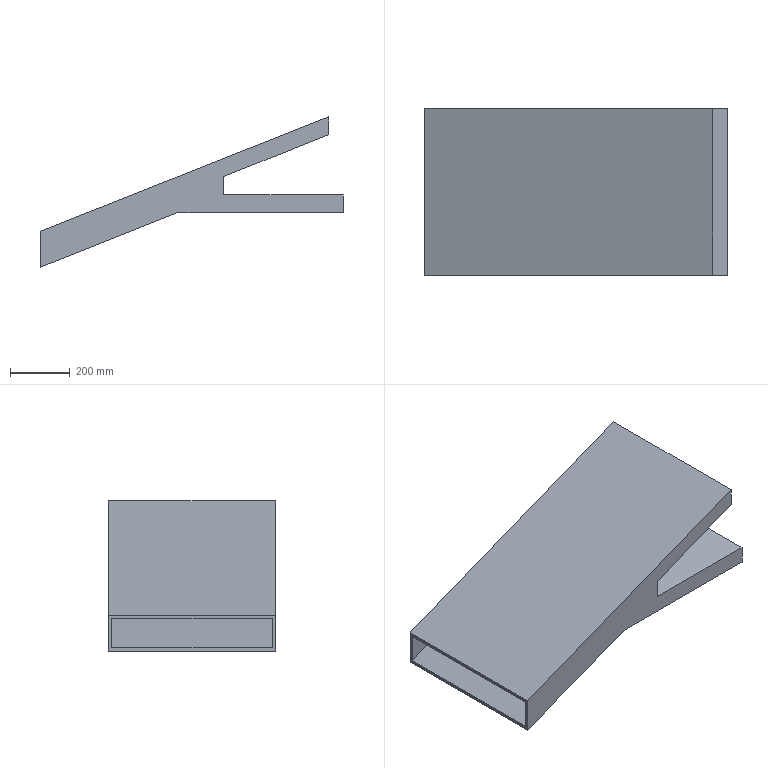Part | SolidWorks | features Extrusion 1, ICE 1, Shell 1 | 1 solid | 23 faces | box 1012 x 556 x 502.062 mm | volume 17769290 mm3 | plane 23
STEP:
#1=CARTESIAN_POINT('',(500.,0.,0.));
#2=VERTEX_POINT('',#1);
#3=CARTESIAN_POINT('',(500.,0.,-60.));
#4=VERTEX_POINT('',#3);
#5=CARTESIAN_POINT('',(500.,0.,0.));
#6=DIRECTION('',(0.,0.,-1.));
#7=VECTOR('',#6,1000.);
#8=LINE('',#5,#7);
#9=EDGE_CURVE('',#2,#4,#8,.T.);
#10=ORIENTED_EDGE('',*,*,#9,.T.);
#11=CARTESIAN_POINT('',(500.,556.,-60.));
#12=VERTEX_POINT('',#11);
#13=CARTESIAN_POINT('',(500.,556.,-60.));
#14=DIRECTION('',(0.,-1.,0.));
#15=VECTOR('',#14,1000.);
#16=LINE('',#13,#15);
#17=EDGE_CURVE('',#12,#4,#16,.T.);
#18=ORIENTED_EDGE('',*,*,#17,.F.);
#19=CARTESIAN_POINT('',(500.,556.,0.));
#20=VERTEX_POINT('',#19);
#21=CARTESIAN_POINT('',(500.,556.,0.));
#22=DIRECTION('',(0.,0.,-1.));
#23=VECTOR('',#22,1000.);
#24=LINE('',#21,#23);
#25=EDGE_CURVE('',#20,#12,#24,.T.);
#26=ORIENTED_EDGE('',*,*,#25,.F.);
#27=CARTESIAN_POINT('',(500.,556.,0.));
#28=DIRECTION('',(0.,-1.,0.));
#29=VECTOR('',#28,1000.);
#30=LINE('',#27,#29);
#31=EDGE_CURVE('',#20,#2,#30,.T.);
#32=ORIENTED_EDGE('',*,*,#31,.T.);
#33=EDGE_LOOP('',(#10,#18,#26,#32));
#34=FACE_OUTER_BOUND('',#33,.T.);
#35=CARTESIAN_POINT('',(500.,10.,-10.));
#36=VERTEX_POINT('',#35);
#37=CARTESIAN_POINT('',(500.,10.,-50.));
#38=VERTEX_POINT('',#37);
#39=CARTESIAN_POINT('',(500.,10.,0.));
#40=DIRECTION('',(0.,0.,-1.));
#41=VECTOR('',#40,1000.);
#42=LINE('',#39,#41);
#43=EDGE_CURVE('',#36,#38,#42,.T.);
#44=ORIENTED_EDGE('',*,*,#43,.F.);
#45=CARTESIAN_POINT('',(500.,546.,-10.));
#46=VERTEX_POINT('',#45);
#47=CARTESIAN_POINT('',(500.,556.,-10.));
#48=DIRECTION('',(0.,-1.,0.));
#49=VECTOR('',#48,1000.);
#50=LINE('',#47,#49);
#51=EDGE_CURVE('',#46,#36,#50,.T.);
#52=ORIENTED_EDGE('',*,*,#51,.F.);
#53=CARTESIAN_POINT('',(500.,546.,-50.));
#54=VERTEX_POINT('',#53);
#55=CARTESIAN_POINT('',(500.,546.,0.));
#56=DIRECTION('',(0.,0.,-1.));
#57=VECTOR('',#56,1000.);
#58=LINE('',#55,#57);
#59=EDGE_CURVE('',#46,#54,#58,.T.);
#60=ORIENTED_EDGE('',*,*,#59,.T.);
#61=CARTESIAN_POINT('',(500.,556.,-50.));
#62=DIRECTION('',(0.,-1.,0.));
#63=VECTOR('',#62,1000.);
#64=LINE('',#61,#63);
#65=EDGE_CURVE('',#54,#38,#64,.T.);
#66=ORIENTED_EDGE('',*,*,#65,.T.);
#67=EDGE_LOOP('',(#44,#52,#60,#66));
#68=FACE_BOUND('',#67,.T.);
#69=CARTESIAN_POINT('',(500.,556.,0.));
#70=DIRECTION('',(-1.,0.,0.));
#71=DIRECTION('',(0.,0.,1.));
#72=AXIS2_PLACEMENT_3D('',#69,#70,#71);
#73=PLANE('',#72);
#74=ADVANCED_FACE('',(#34,#68),#73,.F.);
#75=CARTESIAN_POINT('',(-511.593,0.,-241.017));
#76=VERTEX_POINT('',#75);
#77=CARTESIAN_POINT('',(-511.593,0.,-121.017));
#78=VERTEX_POINT('',#77);
#79=CARTESIAN_POINT('',(-511.593,0.,-241.017));
#80=DIRECTION('',(0.,0.,1.));
#81=VECTOR('',#80,1000.);
#82=LINE('',#79,#81);
#83=EDGE_CURVE('',#76,#78,#82,.T.);
#84=ORIENTED_EDGE('',*,*,#83,.T.);
#85=CARTESIAN_POINT('',(-511.593,556.,-121.017));
#86=VERTEX_POINT('',#85);
#87=CARTESIAN_POINT('',(-511.593,556.,-121.017));
#88=DIRECTION('',(0.,-1.,0.));
#89=VECTOR('',#88,1000.);
#90=LINE('',#87,#89);
#91=EDGE_CURVE('',#86,#78,#90,.T.);
#92=ORIENTED_EDGE('',*,*,#91,.F.);
#93=CARTESIAN_POINT('',(-511.593,556.,-241.017));
#94=VERTEX_POINT('',#93);
#95=CARTESIAN_POINT('',(-511.593,556.,-241.017));
#96=DIRECTION('',(0.,0.,1.));
#97=VECTOR('',#96,1000.);
#98=LINE('',#95,#97);
#99=EDGE_CURVE('',#94,#86,#98,.T.);
#100=ORIENTED_EDGE('',*,*,#99,.F.);
#101=CARTESIAN_POINT('',(-511.593,556.,-241.017));
#102=DIRECTION('',(0.,-1.,0.));
#103=VECTOR('',#102,1000.);
#104=LINE('',#101,#103);
#105=EDGE_CURVE('',#94,#76,#104,.T.);
#106=ORIENTED_EDGE('',*,*,#105,.T.);
#107=EDGE_LOOP('',(#84,#92,#100,#106));
#108=FACE_OUTER_BOUND('',#107,.T.);
#109=CARTESIAN_POINT('',(-511.593,10.,-230.257));
#110=VERTEX_POINT('',#109);
#111=CARTESIAN_POINT('',(-511.593,10.,-131.777));
#112=VERTEX_POINT('',#111);
#113=CARTESIAN_POINT('',(-511.593,10.,-241.017));
#114=DIRECTION('',(0.,0.,1.));
#115=VECTOR('',#114,1000.);
#116=LINE('',#113,#115);
#117=EDGE_CURVE('',#110,#112,#116,.T.);
#118=ORIENTED_EDGE('',*,*,#117,.F.);
#119=CARTESIAN_POINT('',(-511.593,546.,-230.257));
#120=VERTEX_POINT('',#119);
#121=CARTESIAN_POINT('',(-511.593,556.,-230.257));
#122=DIRECTION('',(0.,-1.,0.));
#123=VECTOR('',#122,1000.);
#124=LINE('',#121,#123);
#125=EDGE_CURVE('',#120,#110,#124,.T.);
#126=ORIENTED_EDGE('',*,*,#125,.F.);
#127=CARTESIAN_POINT('',(-511.593,546.,-131.777));
#128=VERTEX_POINT('',#127);
#129=CARTESIAN_POINT('',(-511.593,546.,-241.017));
#130=DIRECTION('',(0.,0.,1.));
#131=VECTOR('',#130,1000.);
#132=LINE('',#129,#131);
#133=EDGE_CURVE('',#120,#128,#132,.T.);
#134=ORIENTED_EDGE('',*,*,#133,.T.);
#135=CARTESIAN_POINT('',(-511.593,556.,-131.777));
#136=DIRECTION('',(0.,-1.,0.));
#137=VECTOR('',#136,1000.);
#138=LINE('',#135,#137);
#139=EDGE_CURVE('',#128,#112,#138,.T.);
#140=ORIENTED_EDGE('',*,*,#139,.T.);
#141=EDGE_LOOP('',(#118,#126,#134,#140));
#142=FACE_BOUND('',#141,.T.);
#143=CARTESIAN_POINT('',(-511.593,556.,-241.017));
#144=DIRECTION('',(1.,0.,0.));
#145=DIRECTION('',(0.,0.,-1.));
#146=AXIS2_PLACEMENT_3D('',#143,#144,#145);
#147=PLANE('',#146);
#148=ADVANCED_FACE('',(#108,#142),#147,.F.);
#149=CARTESIAN_POINT('',(450.,0.,261.045));
#150=VERTEX_POINT('',#149);
#151=CARTESIAN_POINT('',(450.,0.,201.045));
#152=VERTEX_POINT('',#151);
#153=CARTESIAN_POINT('',(450.,0.,261.045));
#154=DIRECTION('',(0.,0.,-1.));
#155=VECTOR('',#154,1000.);
#156=LINE('',#153,#155);
#157=EDGE_CURVE('',#150,#152,#156,.T.);
#158=ORIENTED_EDGE('',*,*,#157,.T.);
#159=CARTESIAN_POINT('',(450.,556.,201.045));
#160=VERTEX_POINT('',#159);
#161=CARTESIAN_POINT('',(450.,556.,201.045));
#162=DIRECTION('',(0.,-1.,0.));
#163=VECTOR('',#162,1000.);
#164=LINE('',#161,#163);
#165=EDGE_CURVE('',#160,#152,#164,.T.);
#166=ORIENTED_EDGE('',*,*,#165,.F.);
#167=CARTESIAN_POINT('',(450.,556.,261.045));
#168=VERTEX_POINT('',#167);
#169=CARTESIAN_POINT('',(450.,556.,261.045));
#170=DIRECTION('',(0.,0.,-1.));
#171=VECTOR('',#170,1000.);
#172=LINE('',#169,#171);
#173=EDGE_CURVE('',#168,#160,#172,.T.);
#174=ORIENTED_EDGE('',*,*,#173,.F.);
#175=CARTESIAN_POINT('',(450.,556.,261.045));
#176=DIRECTION('',(0.,-1.,0.));
#177=VECTOR('',#176,1000.);
#178=LINE('',#175,#177);
#179=EDGE_CURVE('',#168,#150,#178,.T.);
#180=ORIENTED_EDGE('',*,*,#179,.T.);
#181=EDGE_LOOP('',(#158,#166,#174,#180));
#182=FACE_OUTER_BOUND('',#181,.T.);
#183=CARTESIAN_POINT('',(450.,10.,250.284));
#184=VERTEX_POINT('',#183);
#185=CARTESIAN_POINT('',(450.,10.,211.805));
#186=VERTEX_POINT('',#185);
#187=CARTESIAN_POINT('',(450.,10.,261.045));
#188=DIRECTION('',(0.,0.,-1.));
#189=VECTOR('',#188,1000.);
#190=LINE('',#187,#189);
#191=EDGE_CURVE('',#184,#186,#190,.T.);
#192=ORIENTED_EDGE('',*,*,#191,.F.);
#193=CARTESIAN_POINT('',(450.,546.,250.284));
#194=VERTEX_POINT('',#193);
#195=CARTESIAN_POINT('',(450.,556.,250.284));
#196=DIRECTION('',(0.,-1.,0.));
#197=VECTOR('',#196,1000.);
#198=LINE('',#195,#197);
#199=EDGE_CURVE('',#194,#184,#198,.T.);
#200=ORIENTED_EDGE('',*,*,#199,.F.);
#201=CARTESIAN_POINT('',(450.,546.,211.805));
#202=VERTEX_POINT('',#201);
#203=CARTESIAN_POINT('',(450.,546.,261.045));
#204=DIRECTION('',(0.,0.,-1.));
#205=VECTOR('',#204,1000.);
#206=LINE('',#203,#205);
#207=EDGE_CURVE('',#194,#202,#206,.T.);
#208=ORIENTED_EDGE('',*,*,#207,.T.);
#209=CARTESIAN_POINT('',(450.,556.,211.805));
#210=DIRECTION('',(0.,-1.,0.));
#211=VECTOR('',#210,1000.);
#212=LINE('',#209,#211);
#213=EDGE_CURVE('',#202,#186,#212,.T.);
#214=ORIENTED_EDGE('',*,*,#213,.T.);
#215=EDGE_LOOP('',(#192,#200,#208,#214));
#216=FACE_BOUND('',#215,.T.);
#217=CARTESIAN_POINT('',(450.,556.,261.045));
#218=DIRECTION('',(-1.,0.,0.));
#219=DIRECTION('',(0.,0.,1.));
#220=AXIS2_PLACEMENT_3D('',#217,#218,#219);
#221=PLANE('',#220);
#222=ADVANCED_FACE('',(#182,#216),#221,.F.);
#223=CARTESIAN_POINT('',(-56.,41.096,-60.));
#224=VERTEX_POINT('',#223);
#225=CARTESIAN_POINT('',(-56.,0.,-60.));
#226=VERTEX_POINT('',#225);
#227=CARTESIAN_POINT('',(-56.,556.,-60.));
#228=DIRECTION('',(0.,-1.,0.));
#229=VECTOR('',#228,1000.);
#230=LINE('',#227,#229);
#231=EDGE_CURVE('',#224,#226,#230,.T.);
#232=ORIENTED_EDGE('',*,*,#231,.F.);
#233=CARTESIAN_POINT('',(44.,41.096,-60.));
#234=VERTEX_POINT('',#233);
#235=CARTESIAN_POINT('',(-56.,41.096,-60.));
#236=DIRECTION('',(-1.,0.,0.));
#237=VECTOR('',#236,1000.);
#238=LINE('',#235,#237);
#239=EDGE_CURVE('',#234,#224,#238,.T.);
#240=ORIENTED_EDGE('',*,*,#239,.F.);
#241=CARTESIAN_POINT('',(44.,485.332,-60.));
#242=VERTEX_POINT('',#241);
#243=CARTESIAN_POINT('',(44.,41.096,-60.));
#244=DIRECTION('',(0.,-1.,0.));
#245=VECTOR('',#244,1000.);
#246=LINE('',#243,#245);
#247=EDGE_CURVE('',#242,#234,#246,.T.);
#248=ORIENTED_EDGE('',*,*,#247,.F.);
#249=CARTESIAN_POINT('',(-56.,485.332,-60.));
#250=VERTEX_POINT('',#249);
#251=CARTESIAN_POINT('',(-56.,485.332,-60.));
#252=DIRECTION('',(1.,0.,0.));
#253=VECTOR('',#252,1000.);
#254=LINE('',#251,#253);
#255=EDGE_CURVE('',#250,#242,#254,.T.);
#256=ORIENTED_EDGE('',*,*,#255,.F.);
#257=CARTESIAN_POINT('',(-56.,556.,-60.));
#258=VERTEX_POINT('',#257);
#259=CARTESIAN_POINT('',(-56.,556.,-60.));
#260=DIRECTION('',(0.,-1.,0.));
#261=VECTOR('',#260,1000.);
#262=LINE('',#259,#261);
#263=EDGE_CURVE('',#258,#250,#262,.T.);
#264=ORIENTED_EDGE('',*,*,#263,.F.);
#265=CARTESIAN_POINT('',(500.,556.,-60.));
#266=DIRECTION('',(-1.,0.,0.));
#267=VECTOR('',#266,1000.);
#268=LINE('',#265,#267);
#269=EDGE_CURVE('',#12,#258,#268,.T.);
#270=ORIENTED_EDGE('',*,*,#269,.F.);
#271=ORIENTED_EDGE('',*,*,#17,.T.);
#272=CARTESIAN_POINT('',(500.,0.,-60.));
#273=DIRECTION('',(-1.,0.,0.));
#274=VECTOR('',#273,1000.);
#275=LINE('',#272,#274);
#276=EDGE_CURVE('',#4,#226,#275,.T.);
#277=ORIENTED_EDGE('',*,*,#276,.T.);
#278=EDGE_LOOP('',(#232,#240,#248,#256,#264,#270,#271,#277));
#279=FACE_OUTER_BOUND('',#278,.T.);
#280=CARTESIAN_POINT('',(500.,556.,-60.));
#281=DIRECTION('',(0.,0.,1.));
#282=DIRECTION('',(1.,0.,0.));
#283=AXIS2_PLACEMENT_3D('',#280,#281,#282);
#284=PLANE('',#283);
#285=ADVANCED_FACE('',(#279),#284,.F.);
#286=CARTESIAN_POINT('',(-56.,0.,-60.));
#287=DIRECTION('',(-0.9293,0.,-0.3692));
#288=VECTOR('',#287,1000.);
#289=LINE('',#286,#288);
#290=EDGE_CURVE('',#226,#76,#289,.T.);
#291=ORIENTED_EDGE('',*,*,#290,.T.);
#292=ORIENTED_EDGE('',*,*,#105,.F.);
#293=CARTESIAN_POINT('',(-56.,556.,-60.));
#294=DIRECTION('',(-0.9293,0.,-0.3692));
#295=VECTOR('',#294,1000.);
#296=LINE('',#293,#295);
#297=EDGE_CURVE('',#258,#94,#296,.T.);
#298=ORIENTED_EDGE('',*,*,#297,.F.);
#299=ORIENTED_EDGE('',*,*,#263,.T.);
#300=CARTESIAN_POINT('',(-56.,41.096,-60.));
#301=DIRECTION('',(0.,1.,0.));
#302=VECTOR('',#301,1000.);
#303=LINE('',#300,#302);
#304=EDGE_CURVE('',#224,#250,#303,.T.);
#305=ORIENTED_EDGE('',*,*,#304,.F.);
#306=ORIENTED_EDGE('',*,*,#231,.T.);
#307=EDGE_LOOP('',(#291,#292,#298,#299,#305,#306));
#308=FACE_OUTER_BOUND('',#307,.T.);
#309=CARTESIAN_POINT('',(-56.,556.,-60.));
#310=DIRECTION('',(-0.3692,0.,0.9293));
#311=DIRECTION('',(0.9293,0.,0.3692));
#312=AXIS2_PLACEMENT_3D('',#309,#310,#311);
#313=PLANE('',#312);
#314=ADVANCED_FACE('',(#308),#313,.F.);
#315=CARTESIAN_POINT('',(-511.593,0.,-121.017));
#316=DIRECTION('',(0.9293,0.,0.3692));
#317=VECTOR('',#316,1000.);
#318=LINE('',#315,#317);
#319=EDGE_CURVE('',#78,#150,#318,.T.);
#320=ORIENTED_EDGE('',*,*,#319,.T.);
#321=ORIENTED_EDGE('',*,*,#179,.F.);
#322=CARTESIAN_POINT('',(-511.593,556.,-121.017));
#323=DIRECTION('',(0.9293,0.,0.3692));
#324=VECTOR('',#323,1000.);
#325=LINE('',#322,#324);
#326=EDGE_CURVE('',#86,#168,#325,.T.);
#327=ORIENTED_EDGE('',*,*,#326,.F.);
#328=ORIENTED_EDGE('',*,*,#91,.T.);
#329=EDGE_LOOP('',(#320,#321,#327,#328));
#330=FACE_OUTER_BOUND('',#329,.T.);
#331=CARTESIAN_POINT('',(-511.593,556.,-121.017));
#332=DIRECTION('',(0.3692,0.,-0.9293));
#333=DIRECTION('',(-0.9293,0.,-0.3692));
#334=AXIS2_PLACEMENT_3D('',#331,#332,#333);
#335=PLANE('',#334);
#336=ADVANCED_FACE('',(#330),#335,.F.);
#337=CARTESIAN_POINT('',(100.,0.,61.982));
#338=VERTEX_POINT('',#337);
#339=CARTESIAN_POINT('',(450.,0.,201.045));
#340=DIRECTION('',(-0.9293,0.,-0.3692));
#341=VECTOR('',#340,1000.);
#342=LINE('',#339,#341);
#343=EDGE_CURVE('',#152,#338,#342,.T.);
#344=ORIENTED_EDGE('',*,*,#343,.T.);
#345=CARTESIAN_POINT('',(100.,556.,61.982));
#346=VERTEX_POINT('',#345);
#347=CARTESIAN_POINT('',(100.,556.,61.982));
#348=DIRECTION('',(0.,-1.,0.));
#349=VECTOR('',#348,1000.);
#350=LINE('',#347,#349);
#351=EDGE_CURVE('',#346,#338,#350,.T.);
#352=ORIENTED_EDGE('',*,*,#351,.F.);
#353=CARTESIAN_POINT('',(450.,556.,201.045));
#354=DIRECTION('',(-0.9293,0.,-0.3692));
#355=VECTOR('',#354,1000.);
#356=LINE('',#353,#355);
#357=EDGE_CURVE('',#160,#346,#356,.T.);
#358=ORIENTED_EDGE('',*,*,#357,.F.);
#359=ORIENTED_EDGE('',*,*,#165,.T.);
#360=EDGE_LOOP('',(#344,#352,#358,#359));
#361=FACE_OUTER_BOUND('',#360,.T.);
#362=CARTESIAN_POINT('',(450.,556.,201.045));
#363=DIRECTION('',(-0.3692,0.,0.9293));
#364=DIRECTION('',(0.9293,0.,0.3692));
#365=AXIS2_PLACEMENT_3D('',#362,#363,#364);
#366=PLANE('',#365);
#367=ADVANCED_FACE('',(#361),#366,.F.);
#368=CARTESIAN_POINT('',(100.,0.,0.));
#369=VERTEX_POINT('',#368);
#370=CARTESIAN_POINT('',(100.,0.,0.));
#371=DIRECTION('',(0.,0.,-1.));
#372=VECTOR('',#371,1000.);
#373=LINE('',#370,#372);
#374=EDGE_CURVE('',#338,#369,#373,.T.);
#375=ORIENTED_EDGE('',*,*,#374,.T.);
#376=CARTESIAN_POINT('',(100.,556.,0.));
#377=VERTEX_POINT('',#376);
#378=CARTESIAN_POINT('',(100.,556.,0.));
#379=DIRECTION('',(0.,-1.,0.));
#380=VECTOR('',#379,1000.);
#381=LINE('',#378,#380);
#382=EDGE_CURVE('',#377,#369,#381,.T.);
#383=ORIENTED_EDGE('',*,*,#382,.F.);
#384=CARTESIAN_POINT('',(100.,556.,0.));
#385=DIRECTION('',(0.,0.,-1.));
#386=VECTOR('',#385,1000.);
#387=LINE('',#384,#386);
#388=EDGE_CURVE('',#346,#377,#387,.T.);
#389=ORIENTED_EDGE('',*,*,#388,.F.);
#390=ORIENTED_EDGE('',*,*,#351,.T.);
#391=EDGE_LOOP('',(#375,#383,#389,#390));
#392=FACE_OUTER_BOUND('',#391,.T.);
#393=CARTESIAN_POINT('',(100.,556.,0.));
#394=DIRECTION('',(-1.,0.,0.));
#395=DIRECTION('',(0.,0.,1.));
#396=AXIS2_PLACEMENT_3D('',#393,#394,#395);
#397=PLANE('',#396);
#398=ADVANCED_FACE('',(#392),#397,.F.);
#399=CARTESIAN_POINT('',(100.,0.,0.));
#400=DIRECTION('',(1.,0.,0.));
#401=VECTOR('',#400,1000.);
#402=LINE('',#399,#401);
#403=EDGE_CURVE('',#369,#2,#402,.T.);
#404=ORIENTED_EDGE('',*,*,#403,.T.);
#405=ORIENTED_EDGE('',*,*,#31,.F.);
#406=CARTESIAN_POINT('',(100.,556.,0.));
#407=DIRECTION('',(1.,0.,0.));
#408=VECTOR('',#407,1000.);
#409=LINE('',#406,#408);
#410=EDGE_CURVE('',#377,#20,#409,.T.);
#411=ORIENTED_EDGE('',*,*,#410,.F.);
#412=ORIENTED_EDGE('',*,*,#382,.T.);
#413=EDGE_LOOP('',(#404,#405,#411,#412));
#414=FACE_OUTER_BOUND('',#413,.T.);
#415=CARTESIAN_POINT('',(100.,556.,0.));
#416=DIRECTION('',(0.,0.,-1.));
#417=DIRECTION('',(-1.,0.,0.));
#418=AXIS2_PLACEMENT_3D('',#415,#416,#417);
#419=PLANE('',#418);
#420=ADVANCED_FACE('',(#414),#419,.F.);
#421=ORIENTED_EDGE('',*,*,#25,.T.);
#422=ORIENTED_EDGE('',*,*,#269,.T.);
#423=ORIENTED_EDGE('',*,*,#297,.T.);
#424=ORIENTED_EDGE('',*,*,#99,.T.);
#425=ORIENTED_EDGE('',*,*,#326,.T.);
#426=ORIENTED_EDGE('',*,*,#173,.T.);
#427=ORIENTED_EDGE('',*,*,#357,.T.);
#428=ORIENTED_EDGE('',*,*,#388,.T.);
#429=ORIENTED_EDGE('',*,*,#410,.T.);
#430=EDGE_LOOP('',(#421,#422,#423,#424,#425,#426,#427,#428,#429));
#431=FACE_OUTER_BOUND('',#430,.T.);
#432=CARTESIAN_POINT('',(0.,556.,0.));
#433=DIRECTION('',(0.,1.,0.));
#434=DIRECTION('',(0.,0.,1.));
#435=AXIS2_PLACEMENT_3D('',#432,#433,#434);
#436=PLANE('',#435);
#437=ADVANCED_FACE('',(#431),#436,.T.);
#438=ORIENTED_EDGE('',*,*,#9,.F.);
#439=ORIENTED_EDGE('',*,*,#403,.F.);
#440=ORIENTED_EDGE('',*,*,#374,.F.);
#441=ORIENTED_EDGE('',*,*,#343,.F.);
#442=ORIENTED_EDGE('',*,*,#157,.F.);
#443=ORIENTED_EDGE('',*,*,#319,.F.);
#444=ORIENTED_EDGE('',*,*,#83,.F.);
#445=ORIENTED_EDGE('',*,*,#290,.F.);
#446=ORIENTED_EDGE('',*,*,#276,.F.);
#447=EDGE_LOOP('',(#438,#439,#440,#441,#442,#443,#444,#445,#446));
#448=FACE_OUTER_BOUND('',#447,.T.);
#449=CARTESIAN_POINT('',(0.,0.,0.));
#450=DIRECTION('',(0.,1.,0.));
#451=DIRECTION('',(0.,0.,1.));
#452=AXIS2_PLACEMENT_3D('',#449,#450,#451);
#453=PLANE('',#452);
#454=ADVANCED_FACE('',(#448),#453,.F.);
#455=CARTESIAN_POINT('',(-56.,485.332,-50.));
#456=VERTEX_POINT('',#455);
#457=CARTESIAN_POINT('',(-56.,41.096,-50.));
#458=VERTEX_POINT('',#457);
#459=CARTESIAN_POINT('',(-56.,556.,-50.));
#460=DIRECTION('',(0.,-1.,0.));
#461=VECTOR('',#460,1000.);
#462=LINE('',#459,#461);
#463=EDGE_CURVE('',#456,#458,#462,.T.);
#464=ORIENTED_EDGE('',*,*,#463,.F.);
#465=CARTESIAN_POINT('',(44.,485.332,-50.));
#466=VERTEX_POINT('',#465);
#467=CARTESIAN_POINT('',(500.,485.332,-50.));
#468=DIRECTION('',(-1.,0.,0.));
#469=VECTOR('',#468,1000.);
#470=LINE('',#467,#469);
#471=EDGE_CURVE('',#466,#456,#470,.T.);
#472=ORIENTED_EDGE('',*,*,#471,.F.);
#473=CARTESIAN_POINT('',(44.,41.096,-50.));
#474=VERTEX_POINT('',#473);
#475=CARTESIAN_POINT('',(44.,556.,-50.));
#476=DIRECTION('',(0.,1.,0.));
#477=VECTOR('',#476,1000.);
#478=LINE('',#475,#477);
#479=EDGE_CURVE('',#474,#466,#478,.T.);
#480=ORIENTED_EDGE('',*,*,#479,.F.);
#481=CARTESIAN_POINT('',(500.,41.096,-50.));
#482=DIRECTION('',(1.,0.,0.));
#483=VECTOR('',#482,1000.);
#484=LINE('',#481,#483);
#485=EDGE_CURVE('',#458,#474,#484,.T.);
#486=ORIENTED_EDGE('',*,*,#485,.F.);
#487=EDGE_LOOP('',(#464,#472,#480,#486));
#488=FACE_BOUND('',#487,.T.);
#489=CARTESIAN_POINT('',(-57.914,10.,-50.));
#490=VERTEX_POINT('',#489);
#491=CARTESIAN_POINT('',(500.,10.,-50.));
#492=DIRECTION('',(-1.,0.,0.));
#493=VECTOR('',#492,1000.);
#494=LINE('',#491,#493);
#495=EDGE_CURVE('',#38,#490,#494,.T.);
#496=ORIENTED_EDGE('',*,*,#495,.F.);
#497=ORIENTED_EDGE('',*,*,#65,.F.);
#498=CARTESIAN_POINT('',(-57.914,546.,-50.));
#499=VERTEX_POINT('',#498);
#500=CARTESIAN_POINT('',(500.,546.,-50.));
#501=DIRECTION('',(-1.,0.,0.));
#502=VECTOR('',#501,1000.);
#503=LINE('',#500,#502);
#504=EDGE_CURVE('',#54,#499,#503,.T.);
#505=ORIENTED_EDGE('',*,*,#504,.T.);
#506=CARTESIAN_POINT('',(-57.914,556.,-50.));
#507=DIRECTION('',(0.,-1.,0.));
#508=VECTOR('',#507,1000.);
#509=LINE('',#506,#508);
#510=EDGE_CURVE('',#499,#490,#509,.T.);
#511=ORIENTED_EDGE('',*,*,#510,.T.);
#512=EDGE_LOOP('',(#496,#497,#505,#511));
#513=FACE_OUTER_BOUND('',#512,.T.);
#514=CARTESIAN_POINT('',(500.,556.,-50.));
#515=DIRECTION('',(0.,0.,1.));
#516=DIRECTION('',(1.,0.,0.));
#517=AXIS2_PLACEMENT_3D('',#514,#515,#516);
#518=PLANE('',#517);
#519=ADVANCED_FACE('',(#488,#513),#518,.T.);
#520=CARTESIAN_POINT('',(-59.692,10.,-50.707));
#521=DIRECTION('',(-0.9293,0.,-0.3692));
#522=VECTOR('',#521,1000.);
#523=LINE('',#520,#522);
#524=EDGE_CURVE('',#490,#110,#523,.T.);
#525=ORIENTED_EDGE('',*,*,#524,.F.);
#526=ORIENTED_EDGE('',*,*,#510,.F.);
#527=CARTESIAN_POINT('',(-59.692,546.,-50.707));
#528=DIRECTION('',(-0.9293,0.,-0.3692));
#529=VECTOR('',#528,1000.);
#530=LINE('',#527,#529);
#531=EDGE_CURVE('',#499,#120,#530,.T.);
#532=ORIENTED_EDGE('',*,*,#531,.T.);
#533=ORIENTED_EDGE('',*,*,#125,.T.);
#534=EDGE_LOOP('',(#525,#526,#532,#533));
#535=FACE_OUTER_BOUND('',#534,.T.);
#536=CARTESIAN_POINT('',(-59.692,556.,-50.707));
#537=DIRECTION('',(-0.3692,0.,0.9293));
#538=DIRECTION('',(0.9293,0.,0.3692));
#539=AXIS2_PLACEMENT_3D('',#536,#537,#538);
#540=PLANE('',#539);
#541=ADVANCED_FACE('',(#535),#540,.T.);
#542=CARTESIAN_POINT('',(-507.901,10.,-130.31));
#543=DIRECTION('',(0.9293,0.,0.3692));
#544=VECTOR('',#543,1000.);
#545=LINE('',#542,#544);
#546=EDGE_CURVE('',#112,#184,#545,.T.);
#547=ORIENTED_EDGE('',*,*,#546,.F.);
#548=ORIENTED_EDGE('',*,*,#139,.F.);
#549=CARTESIAN_POINT('',(-507.901,546.,-130.31));
#550=DIRECTION('',(0.9293,0.,0.3692));
#551=VECTOR('',#550,1000.);
#552=LINE('',#549,#551);
#553=EDGE_CURVE('',#128,#194,#552,.T.);
#554=ORIENTED_EDGE('',*,*,#553,.T.);
#555=ORIENTED_EDGE('',*,*,#199,.T.);
#556=EDGE_LOOP('',(#547,#548,#554,#555));
#557=FACE_OUTER_BOUND('',#556,.T.);
#558=CARTESIAN_POINT('',(-507.901,556.,-130.31));
#559=DIRECTION('',(0.3692,0.,-0.9293));
#560=DIRECTION('',(-0.9293,0.,-0.3692));
#561=AXIS2_PLACEMENT_3D('',#558,#559,#560);
#562=PLANE('',#561);
#563=ADVANCED_FACE('',(#557),#562,.T.);
#564=CARTESIAN_POINT('',(90.,10.,68.769));
#565=VERTEX_POINT('',#564);
#566=CARTESIAN_POINT('',(446.308,10.,210.338));
#567=DIRECTION('',(-0.9293,0.,-0.3692));
#568=VECTOR('',#567,1000.);
#569=LINE('',#566,#568);
#570=EDGE_CURVE('',#186,#565,#569,.T.);
#571=ORIENTED_EDGE('',*,*,#570,.F.);
#572=ORIENTED_EDGE('',*,*,#213,.F.);
#573=CARTESIAN_POINT('',(90.,546.,68.769));
#574=VERTEX_POINT('',#573);
#575=CARTESIAN_POINT('',(446.308,546.,210.338));
#576=DIRECTION('',(-0.9293,0.,-0.3692));
#577=VECTOR('',#576,1000.);
#578=LINE('',#575,#577);
#579=EDGE_CURVE('',#202,#574,#578,.T.);
#580=ORIENTED_EDGE('',*,*,#579,.T.);
#581=CARTESIAN_POINT('',(90.,556.,68.769));
#582=DIRECTION('',(0.,-1.,0.));
#583=VECTOR('',#582,1000.);
#584=LINE('',#581,#583);
#585=EDGE_CURVE('',#574,#565,#584,.T.);
#586=ORIENTED_EDGE('',*,*,#585,.T.);
#587=EDGE_LOOP('',(#571,#572,#580,#586));
#588=FACE_OUTER_BOUND('',#587,.T.);
#589=CARTESIAN_POINT('',(446.308,556.,210.338));
#590=DIRECTION('',(-0.3692,0.,0.9293));
#591=DIRECTION('',(0.9293,0.,0.3692));
#592=AXIS2_PLACEMENT_3D('',#589,#590,#591);
#593=PLANE('',#592);
#594=ADVANCED_FACE('',(#588),#593,.T.);
#595=CARTESIAN_POINT('',(90.,10.,-10.));
#596=VERTEX_POINT('',#595);
#597=CARTESIAN_POINT('',(90.,10.,0.));
#598=DIRECTION('',(0.,0.,-1.));
#599=VECTOR('',#598,1000.);
#600=LINE('',#597,#599);
#601=EDGE_CURVE('',#565,#596,#600,.T.);
#602=ORIENTED_EDGE('',*,*,#601,.F.);
#603=ORIENTED_EDGE('',*,*,#585,.F.);
#604=CARTESIAN_POINT('',(90.,546.,-10.));
#605=VERTEX_POINT('',#604);
#606=CARTESIAN_POINT('',(90.,546.,0.));
#607=DIRECTION('',(0.,0.,-1.));
#608=VECTOR('',#607,1000.);
#609=LINE('',#606,#608);
#610=EDGE_CURVE('',#574,#605,#609,.T.);
#611=ORIENTED_EDGE('',*,*,#610,.T.);
#612=CARTESIAN_POINT('',(90.,556.,-10.));
#613=DIRECTION('',(0.,-1.,0.));
#614=VECTOR('',#613,1000.);
#615=LINE('',#612,#614);
#616=EDGE_CURVE('',#605,#596,#615,.T.);
#617=ORIENTED_EDGE('',*,*,#616,.T.);
#618=EDGE_LOOP('',(#602,#603,#611,#617));
#619=FACE_OUTER_BOUND('',#618,.T.);
#620=CARTESIAN_POINT('',(90.,556.,0.));
#621=DIRECTION('',(-1.,0.,0.));
#622=DIRECTION('',(0.,0.,1.));
#623=AXIS2_PLACEMENT_3D('',#620,#621,#622);
#624=PLANE('',#623);
#625=ADVANCED_FACE('',(#619),#624,.T.);
#626=CARTESIAN_POINT('',(100.,10.,-10.));
#627=DIRECTION('',(1.,0.,0.));
#628=VECTOR('',#627,1000.);
#629=LINE('',#626,#628);
#630=EDGE_CURVE('',#596,#36,#629,.T.);
#631=ORIENTED_EDGE('',*,*,#630,.F.);
#632=ORIENTED_EDGE('',*,*,#616,.F.);
#633=CARTESIAN_POINT('',(100.,546.,-10.));
#634=DIRECTION('',(1.,0.,0.));
#635=VECTOR('',#634,1000.);
#636=LINE('',#633,#635);
#637=EDGE_CURVE('',#605,#46,#636,.T.);
#638=ORIENTED_EDGE('',*,*,#637,.T.);
#639=ORIENTED_EDGE('',*,*,#51,.T.);
#640=EDGE_LOOP('',(#631,#632,#638,#639));
#641=FACE_OUTER_BOUND('',#640,.T.);
#642=CARTESIAN_POINT('',(100.,556.,-10.));
#643=DIRECTION('',(0.,0.,-1.));
#644=DIRECTION('',(-1.,0.,0.));
#645=AXIS2_PLACEMENT_3D('',#642,#643,#644);
#646=PLANE('',#645);
#647=ADVANCED_FACE('',(#641),#646,.T.);
#648=ORIENTED_EDGE('',*,*,#59,.F.);
#649=ORIENTED_EDGE('',*,*,#637,.F.);
#650=ORIENTED_EDGE('',*,*,#610,.F.);
#651=ORIENTED_EDGE('',*,*,#579,.F.);
#652=ORIENTED_EDGE('',*,*,#207,.F.);
#653=ORIENTED_EDGE('',*,*,#553,.F.);
#654=ORIENTED_EDGE('',*,*,#133,.F.);
#655=ORIENTED_EDGE('',*,*,#531,.F.);
#656=ORIENTED_EDGE('',*,*,#504,.F.);
#657=EDGE_LOOP('',(#648,#649,#650,#651,#652,#653,#654,#655,#656));
#658=FACE_OUTER_BOUND('',#657,.T.);
#659=CARTESIAN_POINT('',(0.,546.,0.));
#660=DIRECTION('',(0.,1.,0.));
#661=DIRECTION('',(0.,0.,1.));
#662=AXIS2_PLACEMENT_3D('',#659,#660,#661);
#663=PLANE('',#662);
#664=ADVANCED_FACE('',(#658),#663,.F.);
#665=ORIENTED_EDGE('',*,*,#43,.T.);
#666=ORIENTED_EDGE('',*,*,#495,.T.);
#667=ORIENTED_EDGE('',*,*,#524,.T.);
#668=ORIENTED_EDGE('',*,*,#117,.T.);
#669=ORIENTED_EDGE('',*,*,#546,.T.);
#670=ORIENTED_EDGE('',*,*,#191,.T.);
#671=ORIENTED_EDGE('',*,*,#570,.T.);
#672=ORIENTED_EDGE('',*,*,#601,.T.);
#673=ORIENTED_EDGE('',*,*,#630,.T.);
#674=EDGE_LOOP('',(#665,#666,#667,#668,#669,#670,#671,#672,#673));
#675=FACE_OUTER_BOUND('',#674,.T.);
#676=CARTESIAN_POINT('',(0.,10.,0.));
#677=DIRECTION('',(0.,1.,0.));
#678=DIRECTION('',(0.,0.,1.));
#679=AXIS2_PLACEMENT_3D('',#676,#677,#678);
#680=PLANE('',#679);
#681=ADVANCED_FACE('',(#675),#680,.T.);
#682=ORIENTED_EDGE('',*,*,#463,.T.);
#683=CARTESIAN_POINT('',(-56.,41.096,-45.));
#684=DIRECTION('',(0.,0.,-1.));
#685=VECTOR('',#684,1000.);
#686=LINE('',#683,#685);
#687=EDGE_CURVE('',#458,#224,#686,.T.);
#688=ORIENTED_EDGE('',*,*,#687,.T.);
#689=ORIENTED_EDGE('',*,*,#304,.T.);
#690=CARTESIAN_POINT('',(-56.,485.332,-45.));
#691=DIRECTION('',(0.,0.,-1.));
#692=VECTOR('',#691,1000.);
#693=LINE('',#690,#692);
#694=EDGE_CURVE('',#456,#250,#693,.T.);
#695=ORIENTED_EDGE('',*,*,#694,.F.);
#696=EDGE_LOOP('',(#682,#688,#689,#695));
#697=FACE_OUTER_BOUND('',#696,.T.);
#698=CARTESIAN_POINT('',(-56.,41.096,-45.));
#699=DIRECTION('',(-1.,0.,0.));
#700=DIRECTION('',(0.,0.,1.));
#701=AXIS2_PLACEMENT_3D('',#698,#699,#700);
#702=PLANE('',#701);
#703=ADVANCED_FACE('',(#697),#702,.F.);
#704=ORIENTED_EDGE('',*,*,#485,.T.);
#705=CARTESIAN_POINT('',(44.,41.096,-45.));
#706=DIRECTION('',(0.,0.,-1.));
#707=VECTOR('',#706,1000.);
#708=LINE('',#705,#707);
#709=EDGE_CURVE('',#474,#234,#708,.T.);
#710=ORIENTED_EDGE('',*,*,#709,.T.);
#711=ORIENTED_EDGE('',*,*,#239,.T.);
#712=ORIENTED_EDGE('',*,*,#687,.F.);
#713=EDGE_LOOP('',(#704,#710,#711,#712));
#714=FACE_OUTER_BOUND('',#713,.T.);
#715=CARTESIAN_POINT('',(-56.,41.096,-45.));
#716=DIRECTION('',(0.,-1.,0.));
#717=DIRECTION('',(1.,0.,0.));
#718=AXIS2_PLACEMENT_3D('',#715,#716,#717);
#719=PLANE('',#718);
#720=ADVANCED_FACE('',(#714),#719,.F.);
#721=ORIENTED_EDGE('',*,*,#479,.T.);
#722=CARTESIAN_POINT('',(44.,485.332,-45.));
#723=DIRECTION('',(0.,0.,-1.));
#724=VECTOR('',#723,1000.);
#725=LINE('',#722,#724);
#726=EDGE_CURVE('',#466,#242,#725,.T.);
#727=ORIENTED_EDGE('',*,*,#726,.T.);
#728=ORIENTED_EDGE('',*,*,#247,.T.);
#729=ORIENTED_EDGE('',*,*,#709,.F.);
#730=EDGE_LOOP('',(#721,#727,#728,#729));
#731=FACE_OUTER_BOUND('',#730,.T.);
#732=CARTESIAN_POINT('',(44.,41.096,-45.));
#733=DIRECTION('',(1.,0.,0.));
#734=DIRECTION('',(0.,0.,-1.));
#735=AXIS2_PLACEMENT_3D('',#732,#733,#734);
#736=PLANE('',#735);
#737=ADVANCED_FACE('',(#731),#736,.F.);
#738=ORIENTED_EDGE('',*,*,#471,.T.);
#739=ORIENTED_EDGE('',*,*,#694,.T.);
#740=ORIENTED_EDGE('',*,*,#255,.T.);
#741=ORIENTED_EDGE('',*,*,#726,.F.);
#742=EDGE_LOOP('',(#738,#739,#740,#741));
#743=FACE_OUTER_BOUND('',#742,.T.);
#744=CARTESIAN_POINT('',(-56.,485.332,-45.));
#745=DIRECTION('',(0.,1.,0.));
#746=DIRECTION('',(0.,0.,1.));
#747=AXIS2_PLACEMENT_3D('',#744,#745,#746);
#748=PLANE('',#747);
#749=ADVANCED_FACE('',(#743),#748,.F.);
#750=CLOSED_SHELL('',(#74,#148,#222,#285,#314,#336,#367,#398,#420,#437,#454,#519,#541,#563,#594,#625,#647,#664,#681,#703,#720,#737,#749));
#751=MANIFOLD_SOLID_BREP('',#750);
#752=CARTESIAN_POINT('',(0.,0.,0.));
#753=DIRECTION('',(0.,0.,1.));
#754=DIRECTION('',(1.,0.,0.));
#755=AXIS2_PLACEMENT_3D('',#752,#753,#754);
#756=(LENGTH_UNIT()NAMED_UNIT(*)SI_UNIT(.MILLI.,.METRE.));
#757=UNCERTAINTY_MEASURE_WITH_UNIT(LENGTH_MEASURE(0.00001),#756,'','');
#758=(NAMED_UNIT(*)PLANE_ANGLE_UNIT()SI_UNIT($,.RADIAN.));
#759=(NAMED_UNIT(*)SI_UNIT($,.STERADIAN.)SOLID_ANGLE_UNIT());
#760=(GEOMETRIC_REPRESENTATION_CONTEXT(3)GLOBAL_UNCERTAINTY_ASSIGNED_CONTEXT((#757))GLOBAL_UNIT_ASSIGNED_CONTEXT((#756,#758,#759))REPRESENTATION_CONTEXT('',''));
#761=ADVANCED_BREP_SHAPE_REPRESENTATION('',(#751,#755),#760);